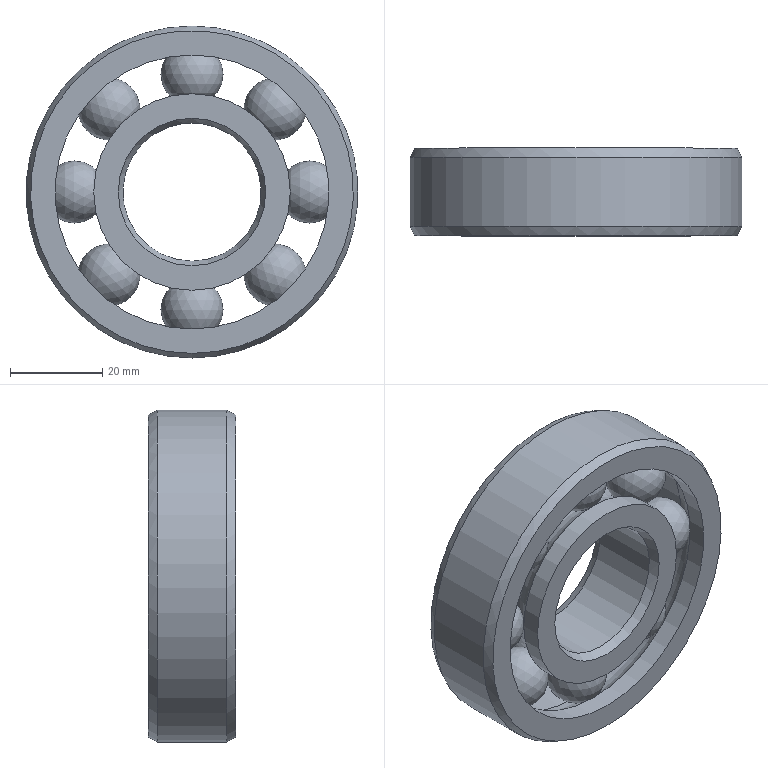Part | NX | features DATUM_CSYS 10, SKETCH 9, SWP104 9, EXTRACT_DATUM_AXIS 8, EXTRACT_DATUM_PLANE 8, EXTRACT_FACE 8, EXTRACT_STRING 8, Instance Feature 7, Pattern Feature 1 | 10 solids | 24 faces | box 72 x 19 x 72 mm | volume 39104 mm3 | sphere 8 | cylinder 6 | plane 4 | cone 4 | torus 2 | commonest cylinder face diameters 42.6 x2 30 x1 59.4 x1 64.5 x1 72 x1
STEP:
#1=CARTESIAN_POINT('',(13.258,9.5,13.258));
#2=VERTEX_POINT('',#1);
#3=VERTEX_LOOP('',#2);
#4=FACE_BOUND('',#3,.T.);
#5=CARTESIAN_POINT('',(18.031,9.5,18.031));
#6=DIRECTION('',(0.7071,0.,0.7071));
#7=DIRECTION('',(0.,1.,0.));
#8=AXIS2_PLACEMENT_3D('',#5,#6,#7);
#9=SPHERICAL_SURFACE('',#8,6.75);
#10=ADVANCED_FACE('',(#4),#9,.T.);
#11=CLOSED_SHELL('',(#10));
#12=MANIFOLD_SOLID_BREP('',#11);
#13=CARTESIAN_POINT('',(-13.258,9.5,-13.258));
#14=VERTEX_POINT('',#13);
#15=VERTEX_LOOP('',#14);
#16=FACE_BOUND('',#15,.T.);
#17=CARTESIAN_POINT('',(-18.031,9.5,-18.031));
#18=DIRECTION('',(-0.7071,0.,-0.7071));
#19=DIRECTION('',(0.,1.,0.));
#20=AXIS2_PLACEMENT_3D('',#17,#18,#19);
#21=SPHERICAL_SURFACE('',#20,6.75);
#22=ADVANCED_FACE('',(#16),#21,.T.);
#23=CLOSED_SHELL('',(#22));
#24=MANIFOLD_SOLID_BREP('',#23);
#25=CARTESIAN_POINT('',(0.,0.,-29.7));
#26=VERTEX_POINT('',#25);
#27=CARTESIAN_POINT('',(0.,0.,0.));
#28=DIRECTION('',(0.,-1.,0.));
#29=DIRECTION('',(0.,0.,-1.));
#30=AXIS2_PLACEMENT_3D('',#27,#28,#29);
#31=CIRCLE('',#30,29.7);
#32=EDGE_CURVE('',#26,#26,#31,.T.);
#33=ORIENTED_EDGE('',*,*,#32,.F.);
#34=EDGE_LOOP('',(#33));
#35=FACE_BOUND('',#34,.T.);
#36=CARTESIAN_POINT('',(0.,0.,-35.));
#37=VERTEX_POINT('',#36);
#38=CARTESIAN_POINT('',(0.,0.,0.));
#39=DIRECTION('',(0.,-1.,0.));
#40=DIRECTION('',(0.,0.,-1.));
#41=AXIS2_PLACEMENT_3D('',#38,#39,#40);
#42=CIRCLE('',#41,35.);
#43=EDGE_CURVE('',#37,#37,#42,.T.);
#44=ORIENTED_EDGE('',*,*,#43,.T.);
#45=EDGE_LOOP('',(#44));
#46=FACE_BOUND('',#45,.T.);
#47=CARTESIAN_POINT('',(0.,0.,35.));
#48=DIRECTION('',(0.,1.,0.));
#49=DIRECTION('',(0.,0.,1.));
#50=AXIS2_PLACEMENT_3D('',#47,#48,#49);
#51=PLANE('',#50);
#52=ADVANCED_FACE('',(#35,#46),#51,.F.);
#53=CARTESIAN_POINT('',(0.,4.216,-29.7));
#54=VERTEX_POINT('',#53);
#55=CARTESIAN_POINT('',(0.,4.216,0.));
#56=DIRECTION('',(0.,-1.,0.));
#57=DIRECTION('',(0.,0.,-1.));
#58=AXIS2_PLACEMENT_3D('',#55,#56,#57);
#59=CIRCLE('',#58,29.7);
#60=EDGE_CURVE('',#54,#54,#59,.T.);
#61=ORIENTED_EDGE('',*,*,#60,.F.);
#62=EDGE_LOOP('',(#61));
#63=FACE_BOUND('',#62,.T.);
#64=ORIENTED_EDGE('',*,*,#32,.T.);
#65=EDGE_LOOP('',(#64));
#66=FACE_BOUND('',#65,.T.);
#67=CARTESIAN_POINT('',(0.,0.,0.));
#68=DIRECTION('',(0.,-1.,0.));
#69=DIRECTION('',(0.,0.,-1.));
#70=AXIS2_PLACEMENT_3D('',#67,#68,#69);
#71=CYLINDRICAL_SURFACE('',#70,29.7);
#72=ADVANCED_FACE('',(#63,#66),#71,.F.);
#73=CARTESIAN_POINT('',(0.,9.5,-32.25));
#74=VERTEX_POINT('',#73);
#75=CARTESIAN_POINT('',(0.,9.5,0.));
#76=DIRECTION('',(0.,-1.,0.));
#77=DIRECTION('',(0.,0.,-1.));
#78=AXIS2_PLACEMENT_3D('',#75,#76,#77);
#79=CIRCLE('',#78,32.25);
#80=EDGE_CURVE('',#74,#74,#79,.T.);
#81=ORIENTED_EDGE('',*,*,#80,.F.);
#82=EDGE_LOOP('',(#81));
#83=FACE_BOUND('',#82,.T.);
#84=ORIENTED_EDGE('',*,*,#60,.T.);
#85=EDGE_LOOP('',(#84));
#86=FACE_BOUND('',#85,.T.);
#87=CARTESIAN_POINT('',(0.,9.5,0.));
#88=DIRECTION('',(0.,-1.,0.));
#89=DIRECTION('',(0.,0.,-1.));
#90=AXIS2_PLACEMENT_3D('',#87,#88,#89);
#91=TOROIDAL_SURFACE('',#90,25.5,6.75);
#92=ADVANCED_FACE('',(#83,#86),#91,.F.);
#93=CARTESIAN_POINT('',(0.,19.,-32.25));
#94=VERTEX_POINT('',#93);
#95=CARTESIAN_POINT('',(0.,19.,0.));
#96=DIRECTION('',(0.,-1.,0.));
#97=DIRECTION('',(0.,0.,-1.));
#98=AXIS2_PLACEMENT_3D('',#95,#96,#97);
#99=CIRCLE('',#98,32.25);
#100=EDGE_CURVE('',#94,#94,#99,.T.);
#101=ORIENTED_EDGE('',*,*,#100,.F.);
#102=EDGE_LOOP('',(#101));
#103=FACE_BOUND('',#102,.T.);
#104=ORIENTED_EDGE('',*,*,#80,.T.);
#105=EDGE_LOOP('',(#104));
#106=FACE_BOUND('',#105,.T.);
#107=CARTESIAN_POINT('',(0.,0.,0.));
#108=DIRECTION('',(0.,-1.,0.));
#109=DIRECTION('',(0.,0.,-1.));
#110=AXIS2_PLACEMENT_3D('',#107,#108,#109);
#111=CYLINDRICAL_SURFACE('',#110,32.25);
#112=ADVANCED_FACE('',(#103,#106),#111,.F.);
#113=CARTESIAN_POINT('',(0.,19.,-35.));
#114=VERTEX_POINT('',#113);
#115=CARTESIAN_POINT('',(0.,19.,0.));
#116=DIRECTION('',(0.,-1.,0.));
#117=DIRECTION('',(0.,0.,-1.));
#118=AXIS2_PLACEMENT_3D('',#115,#116,#117);
#119=CIRCLE('',#118,35.);
#120=EDGE_CURVE('',#114,#114,#119,.T.);
#121=ORIENTED_EDGE('',*,*,#120,.F.);
#122=EDGE_LOOP('',(#121));
#123=FACE_BOUND('',#122,.T.);
#124=ORIENTED_EDGE('',*,*,#100,.T.);
#125=EDGE_LOOP('',(#124));
#126=FACE_BOUND('',#125,.T.);
#127=CARTESIAN_POINT('',(0.,19.,32.25));
#128=DIRECTION('',(0.,-1.,0.));
#129=DIRECTION('',(0.,0.,-1.));
#130=AXIS2_PLACEMENT_3D('',#127,#128,#129);
#131=PLANE('',#130);
#132=ADVANCED_FACE('',(#123,#126),#131,.F.);
#133=CARTESIAN_POINT('',(0.,17.,-36.));
#134=VERTEX_POINT('',#133);
#135=CARTESIAN_POINT('',(0.,17.,0.));
#136=DIRECTION('',(0.,-1.,0.));
#137=DIRECTION('',(0.,0.,-1.));
#138=AXIS2_PLACEMENT_3D('',#135,#136,#137);
#139=CIRCLE('',#138,36.);
#140=EDGE_CURVE('',#134,#134,#139,.T.);
#141=ORIENTED_EDGE('',*,*,#140,.F.);
#142=EDGE_LOOP('',(#141));
#143=FACE_BOUND('',#142,.T.);
#144=ORIENTED_EDGE('',*,*,#120,.T.);
#145=EDGE_LOOP('',(#144));
#146=FACE_BOUND('',#145,.T.);
#147=CARTESIAN_POINT('',(0.,19.,0.));
#148=DIRECTION('',(0.,-1.,0.));
#149=DIRECTION('',(0.,0.,-1.));
#150=AXIS2_PLACEMENT_3D('',#147,#148,#149);
#151=CONICAL_SURFACE('',#150,35.,0.4636);
#152=ADVANCED_FACE('',(#143,#146),#151,.T.);
#153=CARTESIAN_POINT('',(0.,2.,-36.));
#154=VERTEX_POINT('',#153);
#155=CARTESIAN_POINT('',(0.,2.,0.));
#156=DIRECTION('',(0.,-1.,0.));
#157=DIRECTION('',(0.,0.,-1.));
#158=AXIS2_PLACEMENT_3D('',#155,#156,#157);
#159=CIRCLE('',#158,36.);
#160=EDGE_CURVE('',#154,#154,#159,.T.);
#161=ORIENTED_EDGE('',*,*,#160,.F.);
#162=EDGE_LOOP('',(#161));
#163=FACE_BOUND('',#162,.T.);
#164=ORIENTED_EDGE('',*,*,#140,.T.);
#165=EDGE_LOOP('',(#164));
#166=FACE_BOUND('',#165,.T.);
#167=CARTESIAN_POINT('',(0.,0.,0.));
#168=DIRECTION('',(0.,-1.,0.));
#169=DIRECTION('',(0.,0.,-1.));
#170=AXIS2_PLACEMENT_3D('',#167,#168,#169);
#171=CYLINDRICAL_SURFACE('',#170,36.);
#172=ADVANCED_FACE('',(#163,#166),#171,.T.);
#173=ORIENTED_EDGE('',*,*,#43,.F.);
#174=EDGE_LOOP('',(#173));
#175=FACE_BOUND('',#174,.T.);
#176=ORIENTED_EDGE('',*,*,#160,.T.);
#177=EDGE_LOOP('',(#176));
#178=FACE_BOUND('',#177,.T.);
#179=CARTESIAN_POINT('',(0.,2.,0.));
#180=DIRECTION('',(0.,1.,0.));
#181=DIRECTION('',(0.,0.,1.));
#182=AXIS2_PLACEMENT_3D('',#179,#180,#181);
#183=CONICAL_SURFACE('',#182,36.,0.4636);
#184=ADVANCED_FACE('',(#175,#178),#183,.T.);
#185=CLOSED_SHELL('',(#52,#72,#92,#112,#132,#152,#172,#184));
#186=MANIFOLD_SOLID_BREP('',#185);
#187=CARTESIAN_POINT('',(0.,9.5,-18.75));
#188=VERTEX_POINT('',#187);
#189=VERTEX_LOOP('',#188);
#190=FACE_BOUND('',#189,.T.);
#191=CARTESIAN_POINT('',(0.,9.5,-25.5));
#192=DIRECTION('',(0.,0.,-1.));
#193=DIRECTION('',(0.,1.,0.));
#194=AXIS2_PLACEMENT_3D('',#191,#192,#193);
#195=SPHERICAL_SURFACE('',#194,6.75);
#196=ADVANCED_FACE('',(#190),#195,.T.);
#197=CLOSED_SHELL('',(#196));
#198=MANIFOLD_SOLID_BREP('',#197);
#199=CARTESIAN_POINT('',(0.,9.5,18.75));
#200=VERTEX_POINT('',#199);
#201=VERTEX_LOOP('',#200);
#202=FACE_BOUND('',#201,.T.);
#203=CARTESIAN_POINT('',(0.,9.5,25.5));
#204=DIRECTION('',(0.,0.,1.));
#205=DIRECTION('',(0.,1.,0.));
#206=AXIS2_PLACEMENT_3D('',#203,#204,#205);
#207=SPHERICAL_SURFACE('',#206,6.75);
#208=ADVANCED_FACE('',(#202),#207,.T.);
#209=CLOSED_SHELL('',(#208));
#210=MANIFOLD_SOLID_BREP('',#209);
#211=CARTESIAN_POINT('',(13.258,9.5,-13.258));
#212=VERTEX_POINT('',#211);
#213=VERTEX_LOOP('',#212);
#214=FACE_BOUND('',#213,.T.);
#215=CARTESIAN_POINT('',(18.031,9.5,-18.031));
#216=DIRECTION('',(0.7071,0.,-0.7071));
#217=DIRECTION('',(0.,1.,0.));
#218=AXIS2_PLACEMENT_3D('',#215,#216,#217);
#219=SPHERICAL_SURFACE('',#218,6.75);
#220=ADVANCED_FACE('',(#214),#219,.T.);
#221=CLOSED_SHELL('',(#220));
#222=MANIFOLD_SOLID_BREP('',#221);
#223=CARTESIAN_POINT('',(-13.258,9.5,13.258));
#224=VERTEX_POINT('',#223);
#225=VERTEX_LOOP('',#224);
#226=FACE_BOUND('',#225,.T.);
#227=CARTESIAN_POINT('',(-18.031,9.5,18.031));
#228=DIRECTION('',(-0.7071,0.,0.7071));
#229=DIRECTION('',(0.,1.,0.));
#230=AXIS2_PLACEMENT_3D('',#227,#228,#229);
#231=SPHERICAL_SURFACE('',#230,6.75);
#232=ADVANCED_FACE('',(#226),#231,.T.);
#233=CLOSED_SHELL('',(#232));
#234=MANIFOLD_SOLID_BREP('',#233);
#235=CARTESIAN_POINT('',(18.75,9.5,0.));
#236=VERTEX_POINT('',#235);
#237=VERTEX_LOOP('',#236);
#238=FACE_BOUND('',#237,.T.);
#239=CARTESIAN_POINT('',(25.5,9.5,0.));
#240=DIRECTION('',(1.,0.,0.));
#241=DIRECTION('',(0.,1.,0.));
#242=AXIS2_PLACEMENT_3D('',#239,#240,#241);
#243=SPHERICAL_SURFACE('',#242,6.75);
#244=ADVANCED_FACE('',(#238),#243,.T.);
#245=CLOSED_SHELL('',(#244));
#246=MANIFOLD_SOLID_BREP('',#245);
#247=CARTESIAN_POINT('',(-18.75,9.5,0.));
#248=VERTEX_POINT('',#247);
#249=VERTEX_LOOP('',#248);
#250=FACE_BOUND('',#249,.T.);
#251=CARTESIAN_POINT('',(-25.5,9.5,0.));
#252=DIRECTION('',(-1.,0.,0.));
#253=DIRECTION('',(0.,1.,0.));
#254=AXIS2_PLACEMENT_3D('',#251,#252,#253);
#255=SPHERICAL_SURFACE('',#254,6.75);
#256=ADVANCED_FACE('',(#250),#255,.T.);
#257=CLOSED_SHELL('',(#256));
#258=MANIFOLD_SOLID_BREP('',#257);
#259=CARTESIAN_POINT('',(0.,0.,-16.));
#260=VERTEX_POINT('',#259);
#261=CARTESIAN_POINT('',(0.,0.,0.));
#262=DIRECTION('',(0.,-1.,0.));
#263=DIRECTION('',(0.,0.,-1.));
#264=AXIS2_PLACEMENT_3D('',#261,#262,#263);
#265=CIRCLE('',#264,16.);
#266=EDGE_CURVE('',#260,#260,#265,.T.);
#267=ORIENTED_EDGE('',*,*,#266,.F.);
#268=EDGE_LOOP('',(#267));
#269=FACE_BOUND('',#268,.T.);
#270=CARTESIAN_POINT('',(0.,0.,-21.3));
#271=VERTEX_POINT('',#270);
#272=CARTESIAN_POINT('',(0.,0.,0.));
#273=DIRECTION('',(0.,-1.,0.));
#274=DIRECTION('',(0.,0.,-1.));
#275=AXIS2_PLACEMENT_3D('',#272,#273,#274);
#276=CIRCLE('',#275,21.3);
#277=EDGE_CURVE('',#271,#271,#276,.T.);
#278=ORIENTED_EDGE('',*,*,#277,.T.);
#279=EDGE_LOOP('',(#278));
#280=FACE_BOUND('',#279,.T.);
#281=CARTESIAN_POINT('',(0.,0.,21.3));
#282=DIRECTION('',(0.,1.,0.));
#283=DIRECTION('',(0.,0.,1.));
#284=AXIS2_PLACEMENT_3D('',#281,#282,#283);
#285=PLANE('',#284);
#286=ADVANCED_FACE('',(#269,#280),#285,.F.);
#287=CARTESIAN_POINT('',(0.,2.,-15.));
#288=VERTEX_POINT('',#287);
#289=CARTESIAN_POINT('',(0.,2.,0.));
#290=DIRECTION('',(0.,-1.,0.));
#291=DIRECTION('',(0.,0.,-1.));
#292=AXIS2_PLACEMENT_3D('',#289,#290,#291);
#293=CIRCLE('',#292,15.);
#294=EDGE_CURVE('',#288,#288,#293,.T.);
#295=ORIENTED_EDGE('',*,*,#294,.F.);
#296=EDGE_LOOP('',(#295));
#297=FACE_BOUND('',#296,.T.);
#298=ORIENTED_EDGE('',*,*,#266,.T.);
#299=EDGE_LOOP('',(#298));
#300=FACE_BOUND('',#299,.T.);
#301=CARTESIAN_POINT('',(0.,0.,0.));
#302=DIRECTION('',(0.,-1.,0.));
#303=DIRECTION('',(0.,0.,-1.));
#304=AXIS2_PLACEMENT_3D('',#301,#302,#303);
#305=CONICAL_SURFACE('',#304,16.,0.4636);
#306=ADVANCED_FACE('',(#297,#300),#305,.F.);
#307=CARTESIAN_POINT('',(0.,17.,-15.));
#308=VERTEX_POINT('',#307);
#309=CARTESIAN_POINT('',(0.,17.,0.));
#310=DIRECTION('',(0.,-1.,0.));
#311=DIRECTION('',(0.,0.,-1.));
#312=AXIS2_PLACEMENT_3D('',#309,#310,#311);
#313=CIRCLE('',#312,15.);
#314=EDGE_CURVE('',#308,#308,#313,.T.);
#315=ORIENTED_EDGE('',*,*,#314,.F.);
#316=EDGE_LOOP('',(#315));
#317=FACE_BOUND('',#316,.T.);
#318=ORIENTED_EDGE('',*,*,#294,.T.);
#319=EDGE_LOOP('',(#318));
#320=FACE_BOUND('',#319,.T.);
#321=CARTESIAN_POINT('',(0.,0.,0.));
#322=DIRECTION('',(0.,-1.,0.));
#323=DIRECTION('',(0.,0.,-1.));
#324=AXIS2_PLACEMENT_3D('',#321,#322,#323);
#325=CYLINDRICAL_SURFACE('',#324,15.);
#326=ADVANCED_FACE('',(#317,#320),#325,.F.);
#327=CARTESIAN_POINT('',(0.,19.,-16.));
#328=VERTEX_POINT('',#327);
#329=CARTESIAN_POINT('',(0.,19.,0.));
#330=DIRECTION('',(0.,-1.,0.));
#331=DIRECTION('',(0.,0.,-1.));
#332=AXIS2_PLACEMENT_3D('',#329,#330,#331);
#333=CIRCLE('',#332,16.);
#334=EDGE_CURVE('',#328,#328,#333,.T.);
#335=ORIENTED_EDGE('',*,*,#334,.F.);
#336=EDGE_LOOP('',(#335));
#337=FACE_BOUND('',#336,.T.);
#338=ORIENTED_EDGE('',*,*,#314,.T.);
#339=EDGE_LOOP('',(#338));
#340=FACE_BOUND('',#339,.T.);
#341=CARTESIAN_POINT('',(0.,17.,0.));
#342=DIRECTION('',(0.,1.,0.));
#343=DIRECTION('',(0.,0.,1.));
#344=AXIS2_PLACEMENT_3D('',#341,#342,#343);
#345=CONICAL_SURFACE('',#344,15.,0.4636);
#346=ADVANCED_FACE('',(#337,#340),#345,.F.);
#347=CARTESIAN_POINT('',(0.,19.,-21.3));
#348=VERTEX_POINT('',#347);
#349=CARTESIAN_POINT('',(0.,19.,0.));
#350=DIRECTION('',(0.,-1.,0.));
#351=DIRECTION('',(0.,0.,-1.));
#352=AXIS2_PLACEMENT_3D('',#349,#350,#351);
#353=CIRCLE('',#352,21.3);
#354=EDGE_CURVE('',#348,#348,#353,.T.);
#355=ORIENTED_EDGE('',*,*,#354,.F.);
#356=EDGE_LOOP('',(#355));
#357=FACE_BOUND('',#356,.T.);
#358=ORIENTED_EDGE('',*,*,#334,.T.);
#359=EDGE_LOOP('',(#358));
#360=FACE_BOUND('',#359,.T.);
#361=CARTESIAN_POINT('',(0.,19.,16.));
#362=DIRECTION('',(0.,-1.,0.));
#363=DIRECTION('',(0.,0.,-1.));
#364=AXIS2_PLACEMENT_3D('',#361,#362,#363);
#365=PLANE('',#364);
#366=ADVANCED_FACE('',(#357,#360),#365,.F.);
#367=CARTESIAN_POINT('',(0.,14.784,-21.3));
#368=VERTEX_POINT('',#367);
#369=CARTESIAN_POINT('',(0.,14.784,0.));
#370=DIRECTION('',(0.,-1.,0.));
#371=DIRECTION('',(0.,0.,-1.));
#372=AXIS2_PLACEMENT_3D('',#369,#370,#371);
#373=CIRCLE('',#372,21.3);
#374=EDGE_CURVE('',#368,#368,#373,.T.);
#375=ORIENTED_EDGE('',*,*,#374,.F.);
#376=EDGE_LOOP('',(#375));
#377=FACE_BOUND('',#376,.T.);
#378=ORIENTED_EDGE('',*,*,#354,.T.);
#379=EDGE_LOOP('',(#378));
#380=FACE_BOUND('',#379,.T.);
#381=CARTESIAN_POINT('',(0.,0.,0.));
#382=DIRECTION('',(0.,-1.,0.));
#383=DIRECTION('',(0.,0.,-1.));
#384=AXIS2_PLACEMENT_3D('',#381,#382,#383);
#385=CYLINDRICAL_SURFACE('',#384,21.3);
#386=ADVANCED_FACE('',(#377,#380),#385,.T.);
#387=CARTESIAN_POINT('',(0.,4.216,-21.3));
#388=VERTEX_POINT('',#387);
#389=CARTESIAN_POINT('',(0.,4.216,0.));
#390=DIRECTION('',(0.,-1.,0.));
#391=DIRECTION('',(0.,0.,-1.));
#392=AXIS2_PLACEMENT_3D('',#389,#390,#391);
#393=CIRCLE('',#392,21.3);
#394=EDGE_CURVE('',#388,#388,#393,.T.);
#395=ORIENTED_EDGE('',*,*,#394,.F.);
#396=EDGE_LOOP('',(#395));
#397=FACE_BOUND('',#396,.T.);
#398=ORIENTED_EDGE('',*,*,#374,.T.);
#399=EDGE_LOOP('',(#398));
#400=FACE_BOUND('',#399,.T.);
#401=CARTESIAN_POINT('',(0.,9.5,0.));
#402=DIRECTION('',(0.,-1.,0.));
#403=DIRECTION('',(0.,0.,-1.));
#404=AXIS2_PLACEMENT_3D('',#401,#402,#403);
#405=TOROIDAL_SURFACE('',#404,25.5,6.75);
#406=ADVANCED_FACE('',(#397,#400),#405,.F.);
#407=ORIENTED_EDGE('',*,*,#277,.F.);
#408=EDGE_LOOP('',(#407));
#409=FACE_BOUND('',#408,.T.);
#410=ORIENTED_EDGE('',*,*,#394,.T.);
#411=EDGE_LOOP('',(#410));
#412=FACE_BOUND('',#411,.T.);
#413=CARTESIAN_POINT('',(0.,0.,0.));
#414=DIRECTION('',(0.,-1.,0.));
#415=DIRECTION('',(0.,0.,-1.));
#416=AXIS2_PLACEMENT_3D('',#413,#414,#415);
#417=CYLINDRICAL_SURFACE('',#416,21.3);
#418=ADVANCED_FACE('',(#409,#412),#417,.T.);
#419=CLOSED_SHELL('',(#286,#306,#326,#346,#366,#386,#406,#418));
#420=MANIFOLD_SOLID_BREP('',#419);
#421=(LENGTH_UNIT()NAMED_UNIT(*)SI_UNIT(.MILLI.,.METRE.));
#422=UNCERTAINTY_MEASURE_WITH_UNIT(LENGTH_MEASURE(0.00001),#421,'','');
#423=(NAMED_UNIT(*)PLANE_ANGLE_UNIT()SI_UNIT($,.RADIAN.));
#424=(NAMED_UNIT(*)SI_UNIT($,.STERADIAN.)SOLID_ANGLE_UNIT());
#425=(GEOMETRIC_REPRESENTATION_CONTEXT(3)GLOBAL_UNCERTAINTY_ASSIGNED_CONTEXT((#422))GLOBAL_UNIT_ASSIGNED_CONTEXT((#421,#423,#424))REPRESENTATION_CONTEXT('',''));
#426=ADVANCED_BREP_SHAPE_REPRESENTATION('',(#12,#24,#186,#198,#210,#222,#234,#246,#258,#420),#425);